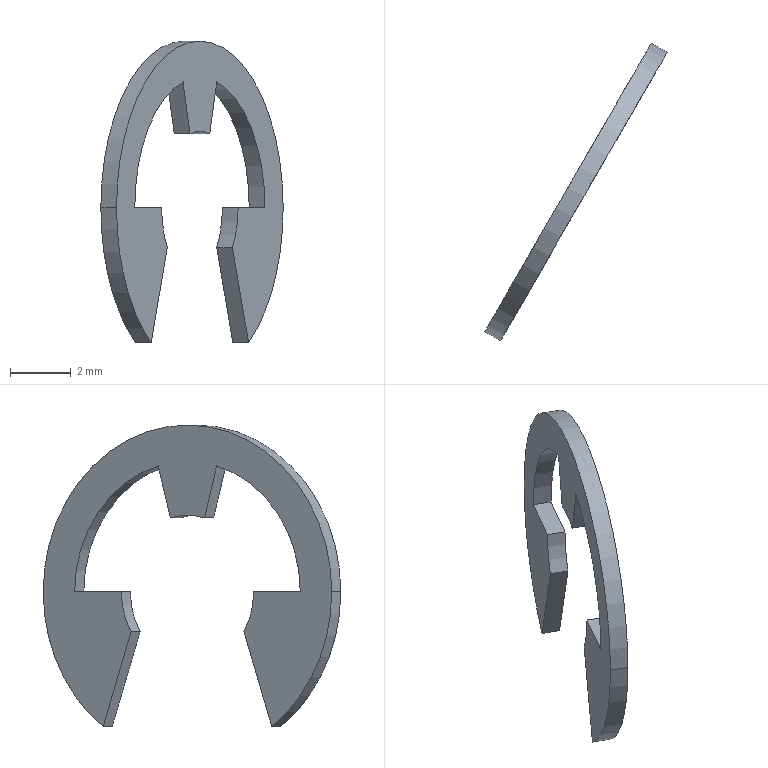Part | SolidWorks | features BaseBody 1 | 1 solid | 16 faces | box 6.02 x 9.826 x 9.962 mm | volume 24.85 mm3 | cylinder 8 | plane 8 | commonest cylinder face diameters 5.05 x3 11 x3 8.6 x2
STEP:
#1=CARTESIAN_POINT('',(-275.187,1817.147,-1178.));
#2=VERTEX_POINT('',#1);
#3=CARTESIAN_POINT('',(-280.687,1807.621,-1178.));
#4=VERTEX_POINT('',#3);
#5=CARTESIAN_POINT('',(-277.937,1812.384,-1178.));
#6=DIRECTION('',(0.866,-0.5,0.));
#7=DIRECTION('',(0.5,0.866,0.));
#8=AXIS2_PLACEMENT_3D('',#5,#6,#7);
#9=CIRCLE('',#8,5.5);
#10=EDGE_CURVE('',#2,#4,#9,.T.);
#11=ORIENTED_EDGE('',*,*,#10,.T.);
#12=CARTESIAN_POINT('',(-280.167,1807.321,-1178.));
#13=VERTEX_POINT('',#12);
#14=CARTESIAN_POINT('',(-280.687,1807.621,-1178.));
#15=DIRECTION('',(0.866,-0.5,0.));
#16=VECTOR('',#15,1000.);
#17=LINE('',#14,#16);
#18=EDGE_CURVE('',#4,#13,#17,.T.);
#19=ORIENTED_EDGE('',*,*,#18,.T.);
#20=CARTESIAN_POINT('',(-274.667,1816.847,-1178.));
#21=VERTEX_POINT('',#20);
#22=CARTESIAN_POINT('',(-277.417,1812.084,-1178.));
#23=DIRECTION('',(-0.866,0.5,0.));
#24=DIRECTION('',(0.5,0.866,0.));
#25=AXIS2_PLACEMENT_3D('',#22,#23,#24);
#26=CIRCLE('',#25,5.5);
#27=EDGE_CURVE('',#13,#21,#26,.T.);
#28=ORIENTED_EDGE('',*,*,#27,.T.);
#29=CARTESIAN_POINT('',(-275.187,1817.147,-1178.));
#30=DIRECTION('',(0.866,-0.5,0.));
#31=VECTOR('',#30,1000.);
#32=LINE('',#29,#31);
#33=EDGE_CURVE('',#2,#21,#32,.T.);
#34=ORIENTED_EDGE('',*,*,#33,.F.);
#35=EDGE_LOOP('',(#11,#19,#28,#34));
#36=FACE_OUTER_BOUND('',#35,.T.);
#37=CARTESIAN_POINT('',(-277.937,1812.384,-1178.));
#38=DIRECTION('',(0.866,-0.5,0.));
#39=DIRECTION('',(0.5,0.866,0.));
#40=AXIS2_PLACEMENT_3D('',#37,#38,#39);
#41=CYLINDRICAL_SURFACE('',#40,5.5);
#42=ADVANCED_FACE('',(#36),#41,.T.);
#43=CARTESIAN_POINT('',(-276.329,1815.169,-1182.462));
#44=VERTEX_POINT('',#43);
#45=CARTESIAN_POINT('',(-277.937,1812.384,-1178.));
#46=DIRECTION('',(0.866,-0.5,0.));
#47=DIRECTION('',(0.5,0.866,0.));
#48=AXIS2_PLACEMENT_3D('',#45,#46,#47);
#49=CIRCLE('',#48,5.5);
#50=EDGE_CURVE('',#44,#2,#49,.T.);
#51=ORIENTED_EDGE('',*,*,#50,.T.);
#52=ORIENTED_EDGE('',*,*,#33,.T.);
#53=CARTESIAN_POINT('',(-275.809,1814.869,-1182.462));
#54=VERTEX_POINT('',#53);
#55=CARTESIAN_POINT('',(-277.417,1812.084,-1178.));
#56=DIRECTION('',(-0.866,0.5,0.));
#57=DIRECTION('',(0.5,0.866,0.));
#58=AXIS2_PLACEMENT_3D('',#55,#56,#57);
#59=CIRCLE('',#58,5.5);
#60=EDGE_CURVE('',#21,#54,#59,.T.);
#61=ORIENTED_EDGE('',*,*,#60,.T.);
#62=CARTESIAN_POINT('',(-276.329,1815.169,-1182.462));
#63=DIRECTION('',(-0.866,0.5,0.));
#64=VECTOR('',#63,1000.);
#65=LINE('',#62,#64);
#66=EDGE_CURVE('',#54,#44,#65,.T.);
#67=ORIENTED_EDGE('',*,*,#66,.T.);
#68=EDGE_LOOP('',(#51,#52,#61,#67));
#69=FACE_OUTER_BOUND('',#68,.T.);
#70=CARTESIAN_POINT('',(-277.937,1812.384,-1178.));
#71=DIRECTION('',(0.866,-0.5,0.));
#72=DIRECTION('',(0.5,0.866,0.));
#73=AXIS2_PLACEMENT_3D('',#70,#71,#72);
#74=CYLINDRICAL_SURFACE('',#73,5.5);
#75=ADVANCED_FACE('',(#69),#74,.T.);
#76=CARTESIAN_POINT('',(-276.342,1813.946,-1179.324));
#77=VERTEX_POINT('',#76);
#78=CARTESIAN_POINT('',(-275.809,1814.869,-1182.462));
#79=DIRECTION('',(-0.1607,-0.2784,0.9469));
#80=VECTOR('',#79,1000.);
#81=LINE('',#78,#80);
#82=EDGE_CURVE('',#54,#77,#81,.T.);
#83=ORIENTED_EDGE('',*,*,#82,.F.);
#84=ORIENTED_EDGE('',*,*,#60,.F.);
#85=ORIENTED_EDGE('',*,*,#27,.F.);
#86=CARTESIAN_POINT('',(-279.025,1809.299,-1182.462));
#87=VERTEX_POINT('',#86);
#88=CARTESIAN_POINT('',(-277.417,1812.084,-1178.));
#89=DIRECTION('',(-0.866,0.5,0.));
#90=DIRECTION('',(0.5,0.866,0.));
#91=AXIS2_PLACEMENT_3D('',#88,#89,#90);
#92=CIRCLE('',#91,5.5);
#93=EDGE_CURVE('',#87,#13,#92,.T.);
#94=ORIENTED_EDGE('',*,*,#93,.F.);
#95=CARTESIAN_POINT('',(-278.492,1810.222,-1179.324));
#96=VERTEX_POINT('',#95);
#97=CARTESIAN_POINT('',(-278.492,1810.222,-1179.324));
#98=DIRECTION('',(-0.1607,-0.2784,-0.9469));
#99=VECTOR('',#98,1000.);
#100=LINE('',#97,#99);
#101=EDGE_CURVE('',#96,#87,#100,.T.);
#102=ORIENTED_EDGE('',*,*,#101,.F.);
#103=CARTESIAN_POINT('',(-278.679,1809.897,-1178.));
#104=VERTEX_POINT('',#103);
#105=CARTESIAN_POINT('',(-277.417,1812.084,-1178.));
#106=DIRECTION('',(0.866,-0.5,0.));
#107=DIRECTION('',(0.5,0.866,0.));
#108=AXIS2_PLACEMENT_3D('',#105,#106,#107);
#109=CIRCLE('',#108,2.525);
#110=EDGE_CURVE('',#104,#96,#109,.T.);
#111=ORIENTED_EDGE('',*,*,#110,.F.);
#112=CARTESIAN_POINT('',(-279.567,1808.36,-1178.));
#113=VERTEX_POINT('',#112);
#114=CARTESIAN_POINT('',(-277.417,1812.084,-1178.));
#115=DIRECTION('',(0.5,0.866,0.));
#116=VECTOR('',#115,1000.);
#117=LINE('',#114,#116);
#118=EDGE_CURVE('',#113,#104,#117,.T.);
#119=ORIENTED_EDGE('',*,*,#118,.F.);
#120=CARTESIAN_POINT('',(-277.973,1811.12,-1173.847));
#121=VERTEX_POINT('',#120);
#122=CARTESIAN_POINT('',(-277.417,1812.084,-1178.));
#123=DIRECTION('',(0.866,-0.5,0.));
#124=DIRECTION('',(0.5,0.866,0.));
#125=AXIS2_PLACEMENT_3D('',#122,#123,#124);
#126=CIRCLE('',#125,4.3);
#127=EDGE_CURVE('',#121,#113,#126,.T.);
#128=ORIENTED_EDGE('',*,*,#127,.F.);
#129=CARTESIAN_POINT('',(-277.744,1811.518,-1175.561));
#130=VERTEX_POINT('',#129);
#131=CARTESIAN_POINT('',(-277.744,1811.518,-1175.561));
#132=DIRECTION('',(-0.1294,-0.2241,0.9659));
#133=VECTOR('',#132,1000.);
#134=LINE('',#131,#133);
#135=EDGE_CURVE('',#130,#121,#134,.T.);
#136=ORIENTED_EDGE('',*,*,#135,.F.);
#137=CARTESIAN_POINT('',(-277.09,1812.65,-1175.561));
#138=VERTEX_POINT('',#137);
#139=CARTESIAN_POINT('',(-277.417,1812.084,-1178.));
#140=DIRECTION('',(0.866,-0.5,0.));
#141=DIRECTION('',(0.5,0.866,0.));
#142=AXIS2_PLACEMENT_3D('',#139,#140,#141);
#143=CIRCLE('',#142,2.525);
#144=EDGE_CURVE('',#138,#130,#143,.T.);
#145=ORIENTED_EDGE('',*,*,#144,.F.);
#146=CARTESIAN_POINT('',(-276.86,1813.048,-1173.847));
#147=VERTEX_POINT('',#146);
#148=CARTESIAN_POINT('',(-276.86,1813.048,-1173.847));
#149=DIRECTION('',(-0.1294,-0.2241,-0.9659));
#150=VECTOR('',#149,1000.);
#151=LINE('',#148,#150);
#152=EDGE_CURVE('',#147,#138,#151,.T.);
#153=ORIENTED_EDGE('',*,*,#152,.F.);
#154=CARTESIAN_POINT('',(-275.267,1815.808,-1178.));
#155=VERTEX_POINT('',#154);
#156=CARTESIAN_POINT('',(-277.417,1812.084,-1178.));
#157=DIRECTION('',(0.866,-0.5,0.));
#158=DIRECTION('',(0.5,0.866,0.));
#159=AXIS2_PLACEMENT_3D('',#156,#157,#158);
#160=CIRCLE('',#159,4.3);
#161=EDGE_CURVE('',#155,#147,#160,.T.);
#162=ORIENTED_EDGE('',*,*,#161,.F.);
#163=CARTESIAN_POINT('',(-276.154,1814.271,-1178.));
#164=VERTEX_POINT('',#163);
#165=CARTESIAN_POINT('',(-277.417,1812.084,-1178.));
#166=DIRECTION('',(0.5,0.866,0.));
#167=VECTOR('',#166,1000.);
#168=LINE('',#165,#167);
#169=EDGE_CURVE('',#164,#155,#168,.T.);
#170=ORIENTED_EDGE('',*,*,#169,.F.);
#171=CARTESIAN_POINT('',(-277.417,1812.084,-1178.));
#172=DIRECTION('',(0.866,-0.5,0.));
#173=DIRECTION('',(0.5,0.866,0.));
#174=AXIS2_PLACEMENT_3D('',#171,#172,#173);
#175=CIRCLE('',#174,2.525);
#176=EDGE_CURVE('',#77,#164,#175,.T.);
#177=ORIENTED_EDGE('',*,*,#176,.F.);
#178=EDGE_LOOP('',(#83,#84,#85,#94,#102,#111,#119,#128,#136,#145,#153,#162,#170,#177));
#179=FACE_OUTER_BOUND('',#178,.T.);
#180=CARTESIAN_POINT('',(-277.417,1812.084,-1178.));
#181=DIRECTION('',(-0.866,0.5,0.));
#182=DIRECTION('',(-0.5,-0.866,0.));
#183=AXIS2_PLACEMENT_3D('',#180,#181,#182);
#184=PLANE('',#183);
#185=ADVANCED_FACE('',(#179),#184,.F.);
#186=CARTESIAN_POINT('',(-276.862,1814.246,-1179.324));
#187=VERTEX_POINT('',#186);
#188=CARTESIAN_POINT('',(-276.862,1814.246,-1179.324));
#189=DIRECTION('',(-0.1607,-0.2784,0.9469));
#190=VECTOR('',#189,1000.);
#191=LINE('',#188,#190);
#192=EDGE_CURVE('',#44,#187,#191,.T.);
#193=ORIENTED_EDGE('',*,*,#192,.F.);
#194=ORIENTED_EDGE('',*,*,#66,.F.);
#195=ORIENTED_EDGE('',*,*,#82,.T.);
#196=CARTESIAN_POINT('',(-276.862,1814.246,-1179.324));
#197=DIRECTION('',(0.866,-0.5,0.));
#198=VECTOR('',#197,1000.);
#199=LINE('',#196,#198);
#200=EDGE_CURVE('',#187,#77,#199,.T.);
#201=ORIENTED_EDGE('',*,*,#200,.F.);
#202=EDGE_LOOP('',(#193,#194,#195,#201));
#203=FACE_OUTER_BOUND('',#202,.T.);
#204=CARTESIAN_POINT('',(-276.862,1814.246,-1179.324));
#205=DIRECTION('',(0.4735,0.8201,0.3214));
#206=DIRECTION('',(-0.866,0.5,0.));
#207=AXIS2_PLACEMENT_3D('',#204,#205,#206);
#208=PLANE('',#207);
#209=ADVANCED_FACE('',(#203),#208,.F.);
#210=ORIENTED_EDGE('',*,*,#18,.F.);
#211=CARTESIAN_POINT('',(-279.544,1809.599,-1182.462));
#212=VERTEX_POINT('',#211);
#213=CARTESIAN_POINT('',(-277.937,1812.384,-1178.));
#214=DIRECTION('',(0.866,-0.5,0.));
#215=DIRECTION('',(0.5,0.866,0.));
#216=AXIS2_PLACEMENT_3D('',#213,#214,#215);
#217=CIRCLE('',#216,5.5);
#218=EDGE_CURVE('',#4,#212,#217,.T.);
#219=ORIENTED_EDGE('',*,*,#218,.T.);
#220=CARTESIAN_POINT('',(-279.544,1809.599,-1182.462));
#221=DIRECTION('',(0.866,-0.5,0.));
#222=VECTOR('',#221,1000.);
#223=LINE('',#220,#222);
#224=EDGE_CURVE('',#212,#87,#223,.T.);
#225=ORIENTED_EDGE('',*,*,#224,.T.);
#226=ORIENTED_EDGE('',*,*,#93,.T.);
#227=EDGE_LOOP('',(#210,#219,#225,#226));
#228=FACE_OUTER_BOUND('',#227,.T.);
#229=CARTESIAN_POINT('',(-277.937,1812.384,-1178.));
#230=DIRECTION('',(0.866,-0.5,0.));
#231=DIRECTION('',(0.5,0.866,0.));
#232=AXIS2_PLACEMENT_3D('',#229,#230,#231);
#233=CYLINDRICAL_SURFACE('',#232,5.5);
#234=ADVANCED_FACE('',(#228),#233,.T.);
#235=CARTESIAN_POINT('',(-279.012,1810.522,-1179.324));
#236=VERTEX_POINT('',#235);
#237=CARTESIAN_POINT('',(-279.012,1810.522,-1179.324));
#238=DIRECTION('',(-0.1607,-0.2784,-0.9469));
#239=VECTOR('',#238,1000.);
#240=LINE('',#237,#239);
#241=EDGE_CURVE('',#236,#212,#240,.T.);
#242=ORIENTED_EDGE('',*,*,#241,.F.);
#243=CARTESIAN_POINT('',(-279.012,1810.522,-1179.324));
#244=DIRECTION('',(-0.866,0.5,0.));
#245=VECTOR('',#244,1000.);
#246=LINE('',#243,#245);
#247=EDGE_CURVE('',#96,#236,#246,.T.);
#248=ORIENTED_EDGE('',*,*,#247,.F.);
#249=ORIENTED_EDGE('',*,*,#101,.T.);
#250=ORIENTED_EDGE('',*,*,#224,.F.);
#251=EDGE_LOOP('',(#242,#248,#249,#250));
#252=FACE_OUTER_BOUND('',#251,.T.);
#253=CARTESIAN_POINT('',(-279.012,1810.522,-1179.324));
#254=DIRECTION('',(-0.4735,-0.8201,0.3214));
#255=DIRECTION('',(0.866,-0.5,0.));
#256=AXIS2_PLACEMENT_3D('',#253,#254,#255);
#257=PLANE('',#256);
#258=ADVANCED_FACE('',(#252),#257,.F.);
#259=CARTESIAN_POINT('',(-279.199,1810.197,-1178.));
#260=VERTEX_POINT('',#259);
#261=CARTESIAN_POINT('',(-277.937,1812.384,-1178.));
#262=DIRECTION('',(0.866,-0.5,0.));
#263=DIRECTION('',(0.5,0.866,0.));
#264=AXIS2_PLACEMENT_3D('',#261,#262,#263);
#265=CIRCLE('',#264,2.525);
#266=EDGE_CURVE('',#260,#236,#265,.T.);
#267=ORIENTED_EDGE('',*,*,#266,.F.);
#268=CARTESIAN_POINT('',(-279.199,1810.197,-1178.));
#269=DIRECTION('',(-0.866,0.5,0.));
#270=VECTOR('',#269,1000.);
#271=LINE('',#268,#270);
#272=EDGE_CURVE('',#104,#260,#271,.T.);
#273=ORIENTED_EDGE('',*,*,#272,.F.);
#274=ORIENTED_EDGE('',*,*,#110,.T.);
#275=ORIENTED_EDGE('',*,*,#247,.T.);
#276=EDGE_LOOP('',(#267,#273,#274,#275));
#277=FACE_OUTER_BOUND('',#276,.T.);
#278=CARTESIAN_POINT('',(-277.937,1812.384,-1178.));
#279=DIRECTION('',(0.866,-0.5,0.));
#280=DIRECTION('',(0.5,0.866,0.));
#281=AXIS2_PLACEMENT_3D('',#278,#279,#280);
#282=CYLINDRICAL_SURFACE('',#281,2.525);
#283=ADVANCED_FACE('',(#277),#282,.F.);
#284=CARTESIAN_POINT('',(-280.087,1808.66,-1178.));
#285=VERTEX_POINT('',#284);
#286=CARTESIAN_POINT('',(-280.087,1808.66,-1178.));
#287=DIRECTION('',(0.5,0.866,0.));
#288=VECTOR('',#287,1000.);
#289=LINE('',#286,#288);
#290=EDGE_CURVE('',#285,#260,#289,.T.);
#291=ORIENTED_EDGE('',*,*,#290,.F.);
#292=CARTESIAN_POINT('',(-279.567,1808.36,-1178.));
#293=DIRECTION('',(-0.866,0.5,0.));
#294=VECTOR('',#293,1000.);
#295=LINE('',#292,#294);
#296=EDGE_CURVE('',#113,#285,#295,.T.);
#297=ORIENTED_EDGE('',*,*,#296,.F.);
#298=ORIENTED_EDGE('',*,*,#118,.T.);
#299=ORIENTED_EDGE('',*,*,#272,.T.);
#300=EDGE_LOOP('',(#291,#297,#298,#299));
#301=FACE_OUTER_BOUND('',#300,.T.);
#302=CARTESIAN_POINT('',(-279.199,1810.197,-1178.));
#303=DIRECTION('',(0.,0.,-1.));
#304=DIRECTION('',(-1.,0.,0.));
#305=AXIS2_PLACEMENT_3D('',#302,#303,#304);
#306=PLANE('',#305);
#307=ADVANCED_FACE('',(#301),#306,.F.);
#308=CARTESIAN_POINT('',(-278.493,1811.42,-1173.847));
#309=VERTEX_POINT('',#308);
#310=CARTESIAN_POINT('',(-277.937,1812.384,-1178.));
#311=DIRECTION('',(0.866,-0.5,0.));
#312=DIRECTION('',(0.5,0.866,0.));
#313=AXIS2_PLACEMENT_3D('',#310,#311,#312);
#314=CIRCLE('',#313,4.3);
#315=EDGE_CURVE('',#309,#285,#314,.T.);
#316=ORIENTED_EDGE('',*,*,#315,.F.);
#317=CARTESIAN_POINT('',(-278.493,1811.42,-1173.847));
#318=DIRECTION('',(-0.866,0.5,0.));
#319=VECTOR('',#318,1000.);
#320=LINE('',#317,#319);
#321=EDGE_CURVE('',#121,#309,#320,.T.);
#322=ORIENTED_EDGE('',*,*,#321,.F.);
#323=ORIENTED_EDGE('',*,*,#127,.T.);
#324=ORIENTED_EDGE('',*,*,#296,.T.);
#325=EDGE_LOOP('',(#316,#322,#323,#324));
#326=FACE_OUTER_BOUND('',#325,.T.);
#327=CARTESIAN_POINT('',(-277.937,1812.384,-1178.));
#328=DIRECTION('',(0.866,-0.5,0.));
#329=DIRECTION('',(0.5,0.866,0.));
#330=AXIS2_PLACEMENT_3D('',#327,#328,#329);
#331=CYLINDRICAL_SURFACE('',#330,4.3);
#332=ADVANCED_FACE('',(#326),#331,.F.);
#333=CARTESIAN_POINT('',(-278.263,1811.818,-1175.561));
#334=VERTEX_POINT('',#333);
#335=CARTESIAN_POINT('',(-278.493,1811.42,-1173.847));
#336=DIRECTION('',(-0.1294,-0.2241,0.9659));
#337=VECTOR('',#336,1000.);
#338=LINE('',#335,#337);
#339=EDGE_CURVE('',#334,#309,#338,.T.);
#340=ORIENTED_EDGE('',*,*,#339,.F.);
#341=CARTESIAN_POINT('',(-278.263,1811.818,-1175.561));
#342=DIRECTION('',(-0.866,0.5,0.));
#343=VECTOR('',#342,1000.);
#344=LINE('',#341,#343);
#345=EDGE_CURVE('',#130,#334,#344,.T.);
#346=ORIENTED_EDGE('',*,*,#345,.F.);
#347=ORIENTED_EDGE('',*,*,#135,.T.);
#348=ORIENTED_EDGE('',*,*,#321,.T.);
#349=EDGE_LOOP('',(#340,#346,#347,#348));
#350=FACE_OUTER_BOUND('',#349,.T.);
#351=CARTESIAN_POINT('',(-278.493,1811.42,-1173.847));
#352=DIRECTION('',(0.483,0.8365,0.2588));
#353=DIRECTION('',(-0.866,0.5,0.));
#354=AXIS2_PLACEMENT_3D('',#351,#352,#353);
#355=PLANE('',#354);
#356=ADVANCED_FACE('',(#350),#355,.F.);
#357=CARTESIAN_POINT('',(-277.61,1812.95,-1175.561));
#358=VERTEX_POINT('',#357);
#359=CARTESIAN_POINT('',(-277.937,1812.384,-1178.));
#360=DIRECTION('',(0.866,-0.5,0.));
#361=DIRECTION('',(0.5,0.866,0.));
#362=AXIS2_PLACEMENT_3D('',#359,#360,#361);
#363=CIRCLE('',#362,2.525);
#364=EDGE_CURVE('',#358,#334,#363,.T.);
#365=ORIENTED_EDGE('',*,*,#364,.F.);
#366=CARTESIAN_POINT('',(-277.61,1812.95,-1175.561));
#367=DIRECTION('',(-0.866,0.5,0.));
#368=VECTOR('',#367,1000.);
#369=LINE('',#366,#368);
#370=EDGE_CURVE('',#138,#358,#369,.T.);
#371=ORIENTED_EDGE('',*,*,#370,.F.);
#372=ORIENTED_EDGE('',*,*,#144,.T.);
#373=ORIENTED_EDGE('',*,*,#345,.T.);
#374=EDGE_LOOP('',(#365,#371,#372,#373));
#375=FACE_OUTER_BOUND('',#374,.T.);
#376=CARTESIAN_POINT('',(-277.937,1812.384,-1178.));
#377=DIRECTION('',(0.866,-0.5,0.));
#378=DIRECTION('',(0.5,0.866,0.));
#379=AXIS2_PLACEMENT_3D('',#376,#377,#378);
#380=CYLINDRICAL_SURFACE('',#379,2.525);
#381=ADVANCED_FACE('',(#375),#380,.F.);
#382=CARTESIAN_POINT('',(-277.38,1813.348,-1173.847));
#383=VERTEX_POINT('',#382);
#384=CARTESIAN_POINT('',(-277.61,1812.95,-1175.561));
#385=DIRECTION('',(-0.1294,-0.2241,-0.9659));
#386=VECTOR('',#385,1000.);
#387=LINE('',#384,#386);
#388=EDGE_CURVE('',#383,#358,#387,.T.);
#389=ORIENTED_EDGE('',*,*,#388,.F.);
#390=CARTESIAN_POINT('',(-277.38,1813.348,-1173.847));
#391=DIRECTION('',(-0.866,0.5,0.));
#392=VECTOR('',#391,1000.);
#393=LINE('',#390,#392);
#394=EDGE_CURVE('',#147,#383,#393,.T.);
#395=ORIENTED_EDGE('',*,*,#394,.F.);
#396=ORIENTED_EDGE('',*,*,#152,.T.);
#397=ORIENTED_EDGE('',*,*,#370,.T.);
#398=EDGE_LOOP('',(#389,#395,#396,#397));
#399=FACE_OUTER_BOUND('',#398,.T.);
#400=CARTESIAN_POINT('',(-277.61,1812.95,-1175.561));
#401=DIRECTION('',(-0.483,-0.8365,0.2588));
#402=DIRECTION('',(0.866,-0.5,0.));
#403=AXIS2_PLACEMENT_3D('',#400,#401,#402);
#404=PLANE('',#403);
#405=ADVANCED_FACE('',(#399),#404,.F.);
#406=CARTESIAN_POINT('',(-275.787,1816.108,-1178.));
#407=VERTEX_POINT('',#406);
#408=CARTESIAN_POINT('',(-277.937,1812.384,-1178.));
#409=DIRECTION('',(0.866,-0.5,0.));
#410=DIRECTION('',(0.5,0.866,0.));
#411=AXIS2_PLACEMENT_3D('',#408,#409,#410);
#412=CIRCLE('',#411,4.3);
#413=EDGE_CURVE('',#407,#383,#412,.T.);
#414=ORIENTED_EDGE('',*,*,#413,.F.);
#415=CARTESIAN_POINT('',(-275.787,1816.108,-1178.));
#416=DIRECTION('',(-0.866,0.5,0.));
#417=VECTOR('',#416,1000.);
#418=LINE('',#415,#417);
#419=EDGE_CURVE('',#155,#407,#418,.T.);
#420=ORIENTED_EDGE('',*,*,#419,.F.);
#421=ORIENTED_EDGE('',*,*,#161,.T.);
#422=ORIENTED_EDGE('',*,*,#394,.T.);
#423=EDGE_LOOP('',(#414,#420,#421,#422));
#424=FACE_OUTER_BOUND('',#423,.T.);
#425=CARTESIAN_POINT('',(-277.937,1812.384,-1178.));
#426=DIRECTION('',(0.866,-0.5,0.));
#427=DIRECTION('',(0.5,0.866,0.));
#428=AXIS2_PLACEMENT_3D('',#425,#426,#427);
#429=CYLINDRICAL_SURFACE('',#428,4.3);
#430=ADVANCED_FACE('',(#424),#429,.F.);
#431=CARTESIAN_POINT('',(-276.674,1814.571,-1178.));
#432=VERTEX_POINT('',#431);
#433=CARTESIAN_POINT('',(-276.674,1814.571,-1178.));
#434=DIRECTION('',(0.5,0.866,0.));
#435=VECTOR('',#434,1000.);
#436=LINE('',#433,#435);
#437=EDGE_CURVE('',#432,#407,#436,.T.);
#438=ORIENTED_EDGE('',*,*,#437,.F.);
#439=CARTESIAN_POINT('',(-276.154,1814.271,-1178.));
#440=DIRECTION('',(-0.866,0.5,0.));
#441=VECTOR('',#440,1000.);
#442=LINE('',#439,#441);
#443=EDGE_CURVE('',#164,#432,#442,.T.);
#444=ORIENTED_EDGE('',*,*,#443,.F.);
#445=ORIENTED_EDGE('',*,*,#169,.T.);
#446=ORIENTED_EDGE('',*,*,#419,.T.);
#447=EDGE_LOOP('',(#438,#444,#445,#446));
#448=FACE_OUTER_BOUND('',#447,.T.);
#449=CARTESIAN_POINT('',(-276.674,1814.571,-1178.));
#450=DIRECTION('',(0.,0.,-1.));
#451=DIRECTION('',(-1.,0.,0.));
#452=AXIS2_PLACEMENT_3D('',#449,#450,#451);
#453=PLANE('',#452);
#454=ADVANCED_FACE('',(#448),#453,.F.);
#455=CARTESIAN_POINT('',(-277.937,1812.384,-1178.));
#456=DIRECTION('',(0.866,-0.5,0.));
#457=DIRECTION('',(0.5,0.866,0.));
#458=AXIS2_PLACEMENT_3D('',#455,#456,#457);
#459=CIRCLE('',#458,2.525);
#460=EDGE_CURVE('',#187,#432,#459,.T.);
#461=ORIENTED_EDGE('',*,*,#460,.F.);
#462=ORIENTED_EDGE('',*,*,#200,.T.);
#463=ORIENTED_EDGE('',*,*,#176,.T.);
#464=ORIENTED_EDGE('',*,*,#443,.T.);
#465=EDGE_LOOP('',(#461,#462,#463,#464));
#466=FACE_OUTER_BOUND('',#465,.T.);
#467=CARTESIAN_POINT('',(-277.937,1812.384,-1178.));
#468=DIRECTION('',(0.866,-0.5,0.));
#469=DIRECTION('',(0.5,0.866,0.));
#470=AXIS2_PLACEMENT_3D('',#467,#468,#469);
#471=CYLINDRICAL_SURFACE('',#470,2.525);
#472=ADVANCED_FACE('',(#466),#471,.F.);
#473=ORIENTED_EDGE('',*,*,#192,.T.);
#474=ORIENTED_EDGE('',*,*,#460,.T.);
#475=ORIENTED_EDGE('',*,*,#437,.T.);
#476=ORIENTED_EDGE('',*,*,#413,.T.);
#477=ORIENTED_EDGE('',*,*,#388,.T.);
#478=ORIENTED_EDGE('',*,*,#364,.T.);
#479=ORIENTED_EDGE('',*,*,#339,.T.);
#480=ORIENTED_EDGE('',*,*,#315,.T.);
#481=ORIENTED_EDGE('',*,*,#290,.T.);
#482=ORIENTED_EDGE('',*,*,#266,.T.);
#483=ORIENTED_EDGE('',*,*,#241,.T.);
#484=ORIENTED_EDGE('',*,*,#218,.F.);
#485=ORIENTED_EDGE('',*,*,#10,.F.);
#486=ORIENTED_EDGE('',*,*,#50,.F.);
#487=EDGE_LOOP('',(#473,#474,#475,#476,#477,#478,#479,#480,#481,#482,#483,#484,#485,#486));
#488=FACE_OUTER_BOUND('',#487,.T.);
#489=CARTESIAN_POINT('',(-277.937,1812.384,-1178.));
#490=DIRECTION('',(-0.866,0.5,0.));
#491=DIRECTION('',(-0.5,-0.866,0.));
#492=AXIS2_PLACEMENT_3D('',#489,#490,#491);
#493=PLANE('',#492);
#494=ADVANCED_FACE('',(#488),#493,.T.);
#495=CLOSED_SHELL('',(#42,#75,#185,#209,#234,#258,#283,#307,#332,#356,#381,#405,#430,#454,#472,#494));
#496=MANIFOLD_SOLID_BREP('',#495);
#497=CARTESIAN_POINT('',(0.,0.,0.));
#498=DIRECTION('',(0.,0.,1.));
#499=DIRECTION('',(1.,0.,0.));
#500=AXIS2_PLACEMENT_3D('',#497,#498,#499);
#501=(LENGTH_UNIT()NAMED_UNIT(*)SI_UNIT(.MILLI.,.METRE.));
#502=UNCERTAINTY_MEASURE_WITH_UNIT(LENGTH_MEASURE(0.00001),#501,'','');
#503=(NAMED_UNIT(*)PLANE_ANGLE_UNIT()SI_UNIT($,.RADIAN.));
#504=(NAMED_UNIT(*)SI_UNIT($,.STERADIAN.)SOLID_ANGLE_UNIT());
#505=(GEOMETRIC_REPRESENTATION_CONTEXT(3)GLOBAL_UNCERTAINTY_ASSIGNED_CONTEXT((#502))GLOBAL_UNIT_ASSIGNED_CONTEXT((#501,#503,#504))REPRESENTATION_CONTEXT('',''));
#506=ADVANCED_BREP_SHAPE_REPRESENTATION('',(#496,#500),#505);